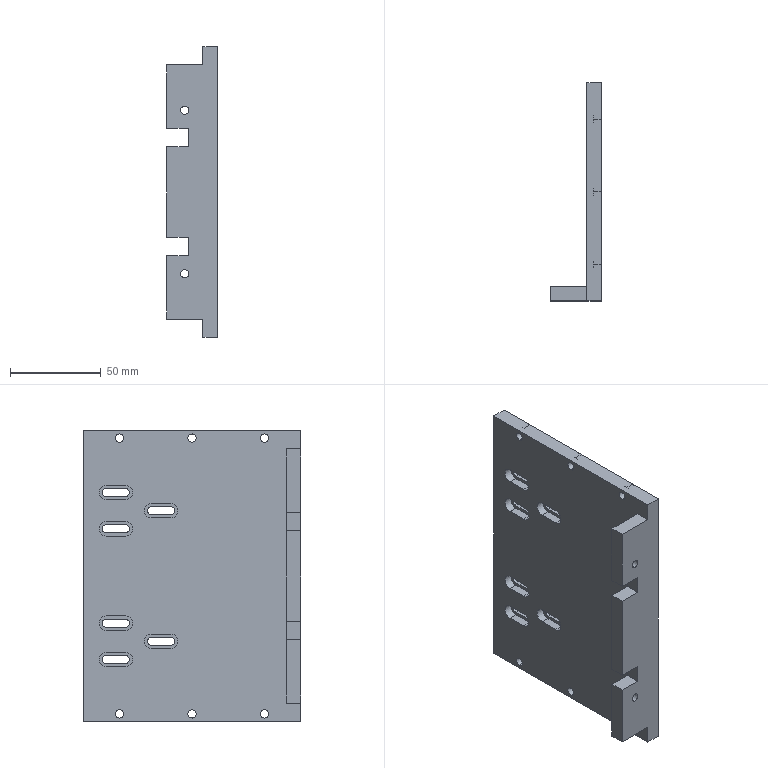Part | SolidWorks | features HoleWzd 4, ICE 3, Extrusion 1 | 1 solid | 112 faces | box 28 x 120 x 160 mm | volume 167009 mm3 | cylinder 56 | plane 56 | commonest cylinder face diameters 4.5 x28 8 x16 7.8 x12